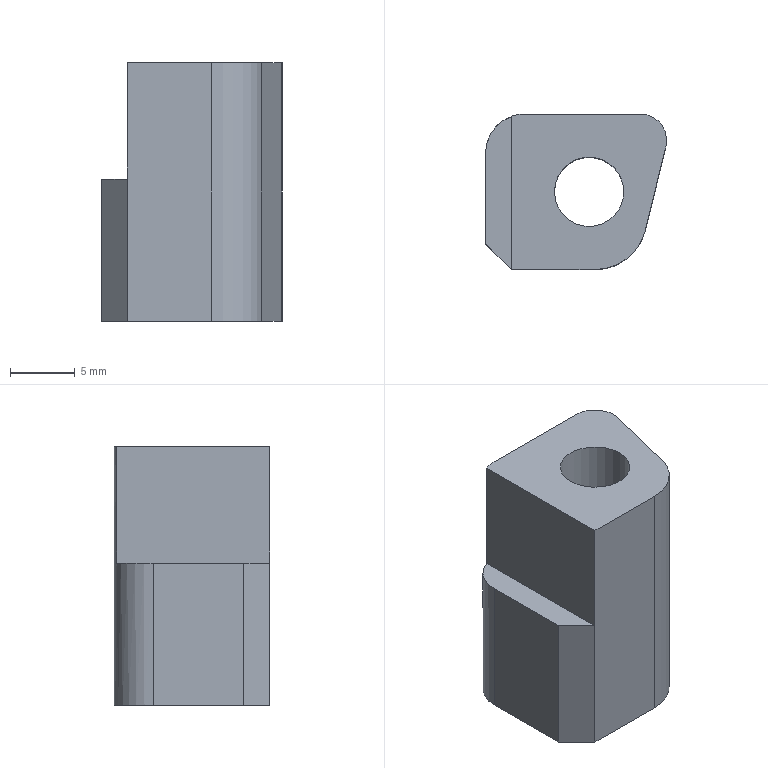Part | STEP file | 1 solid | 14 faces | box 13.98 x 12 x 20 mm | volume 2357 mm3 | plane 9 | cylinder 5 | commonest cylinder face diameters 8 x2 4 x1 5.36 x1 6 x1
STEP:
#1=CARTESIAN_POINT('',(270.135,-42.783,-2.));
#2=VERTEX_POINT('',#1);
#3=CARTESIAN_POINT('',(270.21,-42.397,-2.));
#4=VERTEX_POINT('',#3);
#5=CARTESIAN_POINT('',(266.25,-41.832,-2.));
#6=DIRECTION('',(0.,0.,1.));
#7=DIRECTION('',(1.,0.,0.));
#8=AXIS2_PLACEMENT_3D('',#5,#6,#7);
#9=CIRCLE('',#8,4.);
#10=EDGE_CURVE('',#2,#4,#9,.T.);
#11=ORIENTED_EDGE('',*,*,#10,.T.);
#12=CARTESIAN_POINT('',(268.23,-40.114,-2.));
#13=VERTEX_POINT('',#12);
#14=CARTESIAN_POINT('',(268.23,-42.114,-2.));
#15=DIRECTION('',(0.,0.,1.));
#16=DIRECTION('',(1.,0.,0.));
#17=AXIS2_PLACEMENT_3D('',#14,#15,#16);
#18=CIRCLE('',#17,2.);
#19=EDGE_CURVE('',#4,#13,#18,.T.);
#20=ORIENTED_EDGE('',*,*,#19,.T.);
#21=CARTESIAN_POINT('',(259.25,-40.114,-2.));
#22=VERTEX_POINT('',#21);
#23=CARTESIAN_POINT('',(264.25,-40.114,-2.));
#24=DIRECTION('',(1.,0.,0.));
#25=VECTOR('',#24,1.);
#26=LINE('',#23,#25);
#27=EDGE_CURVE('',#22,#13,#26,.T.);
#28=ORIENTED_EDGE('',*,*,#27,.F.);
#29=CARTESIAN_POINT('',(258.25,-40.286,-2.));
#30=VERTEX_POINT('',#29);
#31=CARTESIAN_POINT('',(259.25,-43.114,-2.));
#32=DIRECTION('',(0.,0.,1.));
#33=DIRECTION('',(1.,0.,0.));
#34=AXIS2_PLACEMENT_3D('',#31,#32,#33);
#35=CIRCLE('',#34,3.);
#36=EDGE_CURVE('',#22,#30,#35,.T.);
#37=ORIENTED_EDGE('',*,*,#36,.T.);
#38=CARTESIAN_POINT('',(258.25,-52.114,-2.));
#39=VERTEX_POINT('',#38);
#40=CARTESIAN_POINT('',(258.25,-46.114,-2.));
#41=DIRECTION('',(0.,1.,0.));
#42=VECTOR('',#41,1.);
#43=LINE('',#40,#42);
#44=EDGE_CURVE('',#39,#30,#43,.T.);
#45=ORIENTED_EDGE('',*,*,#44,.F.);
#46=CARTESIAN_POINT('',(264.711,-52.114,-2.));
#47=VERTEX_POINT('',#46);
#48=CARTESIAN_POINT('',(264.25,-52.114,-2.));
#49=DIRECTION('',(-1.,0.,0.));
#50=VECTOR('',#49,1.);
#51=LINE('',#48,#50);
#52=EDGE_CURVE('',#47,#39,#51,.T.);
#53=ORIENTED_EDGE('',*,*,#52,.F.);
#54=CARTESIAN_POINT('',(268.597,-49.066,-2.));
#55=VERTEX_POINT('',#54);
#56=CARTESIAN_POINT('',(264.711,-48.114,-2.));
#57=DIRECTION('',(0.,0.,1.));
#58=DIRECTION('',(1.,0.,0.));
#59=AXIS2_PLACEMENT_3D('',#56,#57,#58);
#60=CIRCLE('',#59,4.);
#61=EDGE_CURVE('',#47,#55,#60,.T.);
#62=ORIENTED_EDGE('',*,*,#61,.T.);
#63=CARTESIAN_POINT('',(269.033,-47.286,-2.));
#64=DIRECTION('',(0.2379,0.9713,0.));
#65=VECTOR('',#64,1.);
#66=LINE('',#63,#65);
#67=EDGE_CURVE('',#55,#2,#66,.T.);
#68=ORIENTED_EDGE('',*,*,#67,.T.);
#69=EDGE_LOOP('',(#11,#20,#28,#37,#45,#53,#62,#68));
#70=FACE_BOUND('',#69,.T.);
#71=CARTESIAN_POINT('',(266.93,-46.114,-2.));
#72=VERTEX_POINT('',#71);
#73=CARTESIAN_POINT('',(264.25,-46.114,-2.));
#74=DIRECTION('',(0.,0.,-1.));
#75=DIRECTION('',(1.,0.,0.));
#76=AXIS2_PLACEMENT_3D('',#73,#74,#75);
#77=CIRCLE('',#76,2.68);
#78=EDGE_CURVE('',#72,#72,#77,.T.);
#79=ORIENTED_EDGE('',*,*,#78,.T.);
#80=EDGE_LOOP('',(#79));
#81=FACE_BOUND('',#80,.T.);
#82=CARTESIAN_POINT('',(264.25,-46.114,-2.));
#83=DIRECTION('',(0.,0.,1.));
#84=DIRECTION('',(1.,0.,0.));
#85=AXIS2_PLACEMENT_3D('',#82,#83,#84);
#86=PLANE('',#85);
#87=ADVANCED_FACE('',(#70,#81),#86,.T.);
#88=CARTESIAN_POINT('',(258.25,-52.114,-22.));
#89=VERTEX_POINT('',#88);
#90=CARTESIAN_POINT('',(264.711,-52.114,-22.));
#91=VERTEX_POINT('',#90);
#92=CARTESIAN_POINT('',(264.25,-52.114,-22.));
#93=DIRECTION('',(1.,0.,0.));
#94=VECTOR('',#93,1.);
#95=LINE('',#92,#94);
#96=EDGE_CURVE('',#89,#91,#95,.T.);
#97=ORIENTED_EDGE('',*,*,#96,.T.);
#98=CARTESIAN_POINT('',(264.711,-52.114,-22.));
#99=DIRECTION('',(0.,0.,1.));
#100=VECTOR('',#99,1.);
#101=LINE('',#98,#100);
#102=EDGE_CURVE('',#91,#47,#101,.T.);
#103=ORIENTED_EDGE('',*,*,#102,.T.);
#104=ORIENTED_EDGE('',*,*,#52,.T.);
#105=CARTESIAN_POINT('',(258.25,-52.114,-11.));
#106=VERTEX_POINT('',#105);
#107=CARTESIAN_POINT('',(258.25,-52.114,-22.));
#108=DIRECTION('',(0.,0.,1.));
#109=VECTOR('',#108,1.);
#110=LINE('',#107,#109);
#111=EDGE_CURVE('',#106,#39,#110,.T.);
#112=ORIENTED_EDGE('',*,*,#111,.F.);
#113=CARTESIAN_POINT('',(258.25,-52.114,-22.));
#114=DIRECTION('',(0.,0.,-1.));
#115=VECTOR('',#114,1.);
#116=LINE('',#113,#115);
#117=EDGE_CURVE('',#106,#89,#116,.T.);
#118=ORIENTED_EDGE('',*,*,#117,.T.);
#119=EDGE_LOOP('',(#97,#103,#104,#112,#118));
#120=FACE_OUTER_BOUND('',#119,.T.);
#121=CARTESIAN_POINT('',(264.25,-52.114,-22.));
#122=DIRECTION('',(0.,-1.,0.));
#123=DIRECTION('',(0.,0.,-1.));
#124=AXIS2_PLACEMENT_3D('',#121,#122,#123);
#125=PLANE('',#124);
#126=ADVANCED_FACE('',(#120),#125,.T.);
#127=ORIENTED_EDGE('',*,*,#44,.T.);
#128=CARTESIAN_POINT('',(258.25,-40.286,-11.));
#129=VERTEX_POINT('',#128);
#130=CARTESIAN_POINT('',(258.25,-40.286,-2.));
#131=DIRECTION('',(0.,0.,-1.));
#132=VECTOR('',#131,1.);
#133=LINE('',#130,#132);
#134=EDGE_CURVE('',#30,#129,#133,.T.);
#135=ORIENTED_EDGE('',*,*,#134,.T.);
#136=CARTESIAN_POINT('',(258.25,-46.114,-11.));
#137=DIRECTION('',(0.,1.,0.));
#138=VECTOR('',#137,1.);
#139=LINE('',#136,#138);
#140=EDGE_CURVE('',#106,#129,#139,.T.);
#141=ORIENTED_EDGE('',*,*,#140,.F.);
#142=ORIENTED_EDGE('',*,*,#111,.T.);
#143=EDGE_LOOP('',(#127,#135,#141,#142));
#144=FACE_OUTER_BOUND('',#143,.T.);
#145=CARTESIAN_POINT('',(258.25,-46.114,-22.));
#146=DIRECTION('',(-1.,0.,0.));
#147=DIRECTION('',(0.,0.,1.));
#148=AXIS2_PLACEMENT_3D('',#145,#146,#147);
#149=PLANE('',#148);
#150=ADVANCED_FACE('',(#144),#149,.T.);
#151=ORIENTED_EDGE('',*,*,#27,.T.);
#152=CARTESIAN_POINT('',(268.23,-40.114,-22.));
#153=VERTEX_POINT('',#152);
#154=CARTESIAN_POINT('',(268.23,-40.114,-22.));
#155=DIRECTION('',(0.,0.,-1.));
#156=VECTOR('',#155,1.);
#157=LINE('',#154,#156);
#158=EDGE_CURVE('',#13,#153,#157,.T.);
#159=ORIENTED_EDGE('',*,*,#158,.T.);
#160=CARTESIAN_POINT('',(259.25,-40.114,-22.));
#161=VERTEX_POINT('',#160);
#162=CARTESIAN_POINT('',(264.25,-40.114,-22.));
#163=DIRECTION('',(-1.,0.,0.));
#164=VECTOR('',#163,1.);
#165=LINE('',#162,#164);
#166=EDGE_CURVE('',#153,#161,#165,.T.);
#167=ORIENTED_EDGE('',*,*,#166,.T.);
#168=CARTESIAN_POINT('',(259.25,-40.114,-22.));
#169=DIRECTION('',(0.,0.,1.));
#170=VECTOR('',#169,1.);
#171=LINE('',#168,#170);
#172=EDGE_CURVE('',#161,#22,#171,.T.);
#173=ORIENTED_EDGE('',*,*,#172,.T.);
#174=EDGE_LOOP('',(#151,#159,#167,#173));
#175=FACE_OUTER_BOUND('',#174,.T.);
#176=CARTESIAN_POINT('',(264.25,-40.114,-22.));
#177=DIRECTION('',(0.,1.,0.));
#178=DIRECTION('',(0.,0.,1.));
#179=AXIS2_PLACEMENT_3D('',#176,#177,#178);
#180=PLANE('',#179);
#181=ADVANCED_FACE('',(#175),#180,.T.);
#182=ORIENTED_EDGE('',*,*,#166,.F.);
#183=CARTESIAN_POINT('',(270.21,-42.397,-22.));
#184=VERTEX_POINT('',#183);
#185=CARTESIAN_POINT('',(268.23,-42.114,-22.));
#186=DIRECTION('',(0.,0.,-1.));
#187=DIRECTION('',(-1.,0.,0.));
#188=AXIS2_PLACEMENT_3D('',#185,#186,#187);
#189=CIRCLE('',#188,2.);
#190=EDGE_CURVE('',#153,#184,#189,.T.);
#191=ORIENTED_EDGE('',*,*,#190,.T.);
#192=CARTESIAN_POINT('',(270.135,-42.783,-22.));
#193=VERTEX_POINT('',#192);
#194=CARTESIAN_POINT('',(266.25,-41.832,-22.));
#195=DIRECTION('',(0.,0.,-1.));
#196=DIRECTION('',(-1.,0.,0.));
#197=AXIS2_PLACEMENT_3D('',#194,#195,#196);
#198=CIRCLE('',#197,4.);
#199=EDGE_CURVE('',#184,#193,#198,.T.);
#200=ORIENTED_EDGE('',*,*,#199,.T.);
#201=CARTESIAN_POINT('',(268.597,-49.066,-22.));
#202=VERTEX_POINT('',#201);
#203=CARTESIAN_POINT('',(269.033,-47.286,-22.));
#204=DIRECTION('',(-0.2379,-0.9713,0.));
#205=VECTOR('',#204,1.);
#206=LINE('',#203,#205);
#207=EDGE_CURVE('',#193,#202,#206,.T.);
#208=ORIENTED_EDGE('',*,*,#207,.T.);
#209=CARTESIAN_POINT('',(264.711,-48.114,-22.));
#210=DIRECTION('',(0.,0.,-1.));
#211=DIRECTION('',(-1.,0.,0.));
#212=AXIS2_PLACEMENT_3D('',#209,#210,#211);
#213=CIRCLE('',#212,4.);
#214=EDGE_CURVE('',#202,#91,#213,.T.);
#215=ORIENTED_EDGE('',*,*,#214,.T.);
#216=ORIENTED_EDGE('',*,*,#96,.F.);
#217=CARTESIAN_POINT('',(256.25,-50.114,-22.));
#218=VERTEX_POINT('',#217);
#219=CARTESIAN_POINT('',(258.25,-52.114,-22.));
#220=DIRECTION('',(-0.7071,0.7071,0.));
#221=VECTOR('',#220,1.);
#222=LINE('',#219,#221);
#223=EDGE_CURVE('',#89,#218,#222,.T.);
#224=ORIENTED_EDGE('',*,*,#223,.T.);
#225=CARTESIAN_POINT('',(256.25,-43.114,-22.));
#226=VERTEX_POINT('',#225);
#227=CARTESIAN_POINT('',(256.25,-46.114,-22.));
#228=DIRECTION('',(0.,-1.,0.));
#229=VECTOR('',#228,1.);
#230=LINE('',#227,#229);
#231=EDGE_CURVE('',#226,#218,#230,.T.);
#232=ORIENTED_EDGE('',*,*,#231,.F.);
#233=CARTESIAN_POINT('',(259.25,-43.114,-22.));
#234=DIRECTION('',(0.,0.,-1.));
#235=DIRECTION('',(-1.,0.,0.));
#236=AXIS2_PLACEMENT_3D('',#233,#234,#235);
#237=CIRCLE('',#236,3.);
#238=EDGE_CURVE('',#226,#161,#237,.T.);
#239=ORIENTED_EDGE('',*,*,#238,.T.);
#240=EDGE_LOOP('',(#182,#191,#200,#208,#215,#216,#224,#232,#239));
#241=FACE_BOUND('',#240,.T.);
#242=CARTESIAN_POINT('',(261.57,-46.114,-22.));
#243=VERTEX_POINT('',#242);
#244=CARTESIAN_POINT('',(264.25,-46.114,-22.));
#245=DIRECTION('',(0.,0.,-1.));
#246=DIRECTION('',(-1.,0.,0.));
#247=AXIS2_PLACEMENT_3D('',#244,#245,#246);
#248=CIRCLE('',#247,2.68);
#249=EDGE_CURVE('',#243,#243,#248,.T.);
#250=ORIENTED_EDGE('',*,*,#249,.F.);
#251=EDGE_LOOP('',(#250));
#252=FACE_BOUND('',#251,.T.);
#253=CARTESIAN_POINT('',(264.25,-46.114,-22.));
#254=DIRECTION('',(0.,0.,-1.));
#255=DIRECTION('',(-1.,0.,0.));
#256=AXIS2_PLACEMENT_3D('',#253,#254,#255);
#257=PLANE('',#256);
#258=ADVANCED_FACE('',(#241,#252),#257,.T.);
#259=ORIENTED_EDGE('',*,*,#78,.F.);
#260=EDGE_LOOP('',(#259));
#261=FACE_BOUND('',#260,.T.);
#262=ORIENTED_EDGE('',*,*,#249,.T.);
#263=EDGE_LOOP('',(#262));
#264=FACE_BOUND('',#263,.T.);
#265=CARTESIAN_POINT('',(264.25,-46.114,-73.));
#266=DIRECTION('',(0.,0.,1.));
#267=DIRECTION('',(1.,0.,0.));
#268=AXIS2_PLACEMENT_3D('',#265,#266,#267);
#269=CYLINDRICAL_SURFACE('',#268,2.68);
#270=ADVANCED_FACE('',(#261,#264),#269,.F.);
#271=CARTESIAN_POINT('',(256.25,-50.114,-11.));
#272=VERTEX_POINT('',#271);
#273=CARTESIAN_POINT('',(256.25,-43.114,-11.));
#274=VERTEX_POINT('',#273);
#275=CARTESIAN_POINT('',(256.25,-46.114,-11.));
#276=DIRECTION('',(0.,1.,0.));
#277=VECTOR('',#276,1.);
#278=LINE('',#275,#277);
#279=EDGE_CURVE('',#272,#274,#278,.T.);
#280=ORIENTED_EDGE('',*,*,#279,.F.);
#281=CARTESIAN_POINT('',(256.25,-50.114,-11.));
#282=DIRECTION('',(0.7071,-0.7071,0.));
#283=VECTOR('',#282,1.);
#284=LINE('',#281,#283);
#285=EDGE_CURVE('',#272,#106,#284,.T.);
#286=ORIENTED_EDGE('',*,*,#285,.T.);
#287=ORIENTED_EDGE('',*,*,#140,.T.);
#288=CARTESIAN_POINT('',(259.25,-43.114,-11.));
#289=DIRECTION('',(0.,0.,1.));
#290=DIRECTION('',(1.,0.,0.));
#291=AXIS2_PLACEMENT_3D('',#288,#289,#290);
#292=CIRCLE('',#291,3.);
#293=EDGE_CURVE('',#129,#274,#292,.T.);
#294=ORIENTED_EDGE('',*,*,#293,.T.);
#295=EDGE_LOOP('',(#280,#286,#287,#294));
#296=FACE_OUTER_BOUND('',#295,.T.);
#297=CARTESIAN_POINT('',(257.75,-46.114,-11.));
#298=DIRECTION('',(0.,0.,1.));
#299=DIRECTION('',(0.,1.,0.));
#300=AXIS2_PLACEMENT_3D('',#297,#298,#299);
#301=PLANE('',#300);
#302=ADVANCED_FACE('',(#296),#301,.T.);
#303=ORIENTED_EDGE('',*,*,#231,.T.);
#304=CARTESIAN_POINT('',(256.25,-50.114,-22.));
#305=DIRECTION('',(0.,0.,1.));
#306=VECTOR('',#305,1.);
#307=LINE('',#304,#306);
#308=EDGE_CURVE('',#218,#272,#307,.T.);
#309=ORIENTED_EDGE('',*,*,#308,.T.);
#310=ORIENTED_EDGE('',*,*,#279,.T.);
#311=CARTESIAN_POINT('',(256.25,-43.114,-22.));
#312=DIRECTION('',(0.,0.,-1.));
#313=VECTOR('',#312,1.);
#314=LINE('',#311,#313);
#315=EDGE_CURVE('',#274,#226,#314,.T.);
#316=ORIENTED_EDGE('',*,*,#315,.T.);
#317=EDGE_LOOP('',(#303,#309,#310,#316));
#318=FACE_OUTER_BOUND('',#317,.T.);
#319=CARTESIAN_POINT('',(256.25,-46.114,-22.));
#320=DIRECTION('',(-1.,0.,0.));
#321=DIRECTION('',(0.,0.,1.));
#322=AXIS2_PLACEMENT_3D('',#319,#320,#321);
#323=PLANE('',#322);
#324=ADVANCED_FACE('',(#318),#323,.T.);
#325=ORIENTED_EDGE('',*,*,#238,.F.);
#326=ORIENTED_EDGE('',*,*,#315,.F.);
#327=ORIENTED_EDGE('',*,*,#293,.F.);
#328=ORIENTED_EDGE('',*,*,#134,.F.);
#329=ORIENTED_EDGE('',*,*,#36,.F.);
#330=ORIENTED_EDGE('',*,*,#172,.F.);
#331=EDGE_LOOP('',(#325,#326,#327,#328,#329,#330));
#332=FACE_OUTER_BOUND('',#331,.T.);
#333=CARTESIAN_POINT('',(259.25,-43.114,-22.));
#334=DIRECTION('',(0.,0.,1.));
#335=DIRECTION('',(1.,0.,0.));
#336=AXIS2_PLACEMENT_3D('',#333,#334,#335);
#337=CYLINDRICAL_SURFACE('',#336,3.);
#338=ADVANCED_FACE('',(#332),#337,.T.);
#339=ORIENTED_EDGE('',*,*,#223,.F.);
#340=ORIENTED_EDGE('',*,*,#117,.F.);
#341=ORIENTED_EDGE('',*,*,#285,.F.);
#342=ORIENTED_EDGE('',*,*,#308,.F.);
#343=EDGE_LOOP('',(#339,#340,#341,#342));
#344=FACE_OUTER_BOUND('',#343,.T.);
#345=CARTESIAN_POINT('',(256.25,-50.114,-22.));
#346=DIRECTION('',(0.7071,0.7071,0.));
#347=DIRECTION('',(0.,0.,1.));
#348=AXIS2_PLACEMENT_3D('',#345,#346,#347);
#349=PLANE('',#348);
#350=ADVANCED_FACE('',(#344),#349,.F.);
#351=ORIENTED_EDGE('',*,*,#207,.F.);
#352=CARTESIAN_POINT('',(270.135,-42.783,-22.));
#353=DIRECTION('',(0.,0.,1.));
#354=VECTOR('',#353,1.);
#355=LINE('',#352,#354);
#356=EDGE_CURVE('',#193,#2,#355,.T.);
#357=ORIENTED_EDGE('',*,*,#356,.T.);
#358=ORIENTED_EDGE('',*,*,#67,.F.);
#359=CARTESIAN_POINT('',(268.597,-49.066,-22.));
#360=DIRECTION('',(0.,0.,-1.));
#361=VECTOR('',#360,1.);
#362=LINE('',#359,#361);
#363=EDGE_CURVE('',#55,#202,#362,.T.);
#364=ORIENTED_EDGE('',*,*,#363,.T.);
#365=EDGE_LOOP('',(#351,#357,#358,#364));
#366=FACE_OUTER_BOUND('',#365,.T.);
#367=CARTESIAN_POINT('',(267.85,-52.114,-22.));
#368=DIRECTION('',(-0.9713,0.2379,0.));
#369=DIRECTION('',(0.,0.,1.));
#370=AXIS2_PLACEMENT_3D('',#367,#368,#369);
#371=PLANE('',#370);
#372=ADVANCED_FACE('',(#366),#371,.F.);
#373=ORIENTED_EDGE('',*,*,#214,.F.);
#374=ORIENTED_EDGE('',*,*,#363,.F.);
#375=ORIENTED_EDGE('',*,*,#61,.F.);
#376=ORIENTED_EDGE('',*,*,#102,.F.);
#377=EDGE_LOOP('',(#373,#374,#375,#376));
#378=FACE_OUTER_BOUND('',#377,.T.);
#379=CARTESIAN_POINT('',(264.711,-48.114,-22.));
#380=DIRECTION('',(0.,0.,-1.));
#381=DIRECTION('',(-1.,0.,0.));
#382=AXIS2_PLACEMENT_3D('',#379,#380,#381);
#383=CYLINDRICAL_SURFACE('',#382,4.);
#384=ADVANCED_FACE('',(#378),#383,.T.);
#385=ORIENTED_EDGE('',*,*,#199,.F.);
#386=CARTESIAN_POINT('',(270.21,-42.397,-22.));
#387=DIRECTION('',(0.,0.,1.));
#388=VECTOR('',#387,1.);
#389=LINE('',#386,#388);
#390=EDGE_CURVE('',#184,#4,#389,.T.);
#391=ORIENTED_EDGE('',*,*,#390,.T.);
#392=ORIENTED_EDGE('',*,*,#10,.F.);
#393=ORIENTED_EDGE('',*,*,#356,.F.);
#394=EDGE_LOOP('',(#385,#391,#392,#393));
#395=FACE_OUTER_BOUND('',#394,.T.);
#396=CARTESIAN_POINT('',(266.25,-41.832,-22.));
#397=DIRECTION('',(0.,0.,1.));
#398=DIRECTION('',(1.,0.,0.));
#399=AXIS2_PLACEMENT_3D('',#396,#397,#398);
#400=CYLINDRICAL_SURFACE('',#399,4.);
#401=ADVANCED_FACE('',(#395),#400,.T.);
#402=ORIENTED_EDGE('',*,*,#190,.F.);
#403=ORIENTED_EDGE('',*,*,#158,.F.);
#404=ORIENTED_EDGE('',*,*,#19,.F.);
#405=ORIENTED_EDGE('',*,*,#390,.F.);
#406=EDGE_LOOP('',(#402,#403,#404,#405));
#407=FACE_OUTER_BOUND('',#406,.T.);
#408=CARTESIAN_POINT('',(268.23,-42.114,-22.));
#409=DIRECTION('',(0.,0.,1.));
#410=DIRECTION('',(1.,0.,0.));
#411=AXIS2_PLACEMENT_3D('',#408,#409,#410);
#412=CYLINDRICAL_SURFACE('',#411,2.);
#413=ADVANCED_FACE('',(#407),#412,.T.);
#414=CLOSED_SHELL('',(#87,#126,#150,#181,#258,#270,#302,#324,#338,#350,#372,#384,#401,#413));
#415=MANIFOLD_SOLID_BREP('',#414);
#416=(LENGTH_UNIT()NAMED_UNIT(*)SI_UNIT(.MILLI.,.METRE.));
#417=UNCERTAINTY_MEASURE_WITH_UNIT(LENGTH_MEASURE(0.00002),#416,'','');
#418=(NAMED_UNIT(*)PLANE_ANGLE_UNIT()SI_UNIT($,.RADIAN.));
#419=PLANE_ANGLE_MEASURE_WITH_UNIT(PLANE_ANGLE_MEASURE(0.01745),#418);
#420=DIMENSIONAL_EXPONENTS(0.,0.,0.,0.,0.,0.,0.);
#421=(CONVERSION_BASED_UNIT('DEGREE',#419)NAMED_UNIT(#420)PLANE_ANGLE_UNIT());
#422=(NAMED_UNIT(*)SI_UNIT($,.STERADIAN.)SOLID_ANGLE_UNIT());
#423=(GEOMETRIC_REPRESENTATION_CONTEXT(3)GLOBAL_UNCERTAINTY_ASSIGNED_CONTEXT((#417))GLOBAL_UNIT_ASSIGNED_CONTEXT((#416,#421,#422))REPRESENTATION_CONTEXT('',''));
#424=ADVANCED_BREP_SHAPE_REPRESENTATION('',(#415),#423);